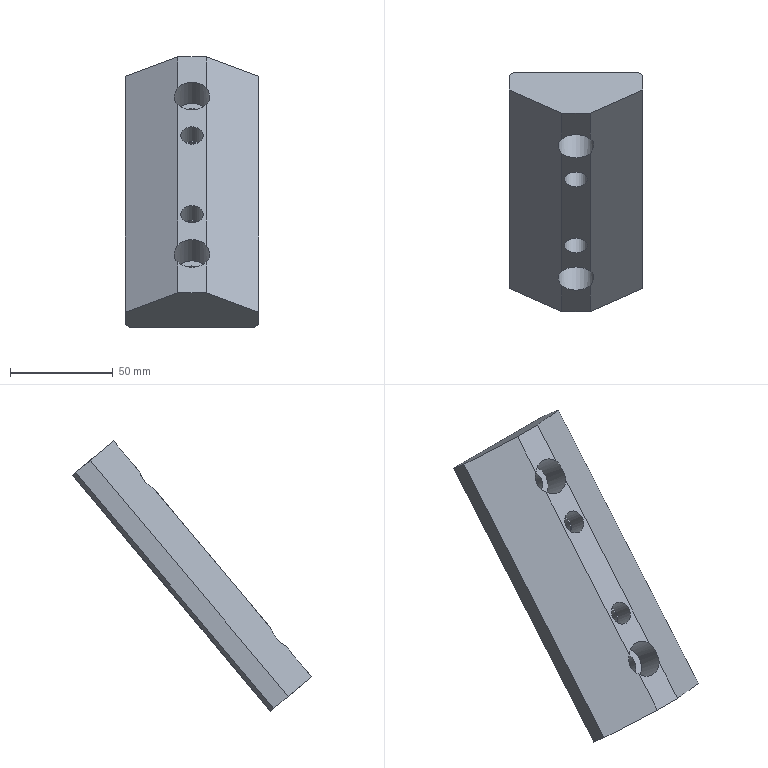Part | NX | features solid 2 | 1 solid | 24 faces | box 65 x 116.335 x 131.619 mm | volume 182247 mm3 | plane 16 | cylinder 8 | commonest cylinder face diameters 11 x4 10 x2 17.5 x2
STEP:
#1=CARTESIAN_POINT('',(-209.428,362.665,-180.748));
#2=VERTEX_POINT('',#1);
#3=CARTESIAN_POINT('',(-195.572,362.665,-180.748));
#4=VERTEX_POINT('',#3);
#5=CARTESIAN_POINT('',(-202.5,366.1,-176.654));
#6=DIRECTION('',(0.,-0.766,0.6428));
#7=DIRECTION('',(0.,0.6428,0.766));
#8=AXIS2_PLACEMENT_3D('',#5,#6,#7);
#9=CIRCLE('',#8,8.75);
#10=EDGE_CURVE('',#2,#4,#9,.T.);
#11=ORIENTED_EDGE('',*,*,#10,.F.);
#12=CARTESIAN_POINT('',(-209.428,350.031,-195.805));
#13=VERTEX_POINT('',#12);
#14=CARTESIAN_POINT('',(-209.428,350.031,-195.805));
#15=DIRECTION('',(0.,0.6428,0.766));
#16=VECTOR('',#15,1000.);
#17=LINE('',#14,#16);
#18=EDGE_CURVE('',#13,#2,#17,.T.);
#19=ORIENTED_EDGE('',*,*,#18,.F.);
#20=CARTESIAN_POINT('',(-195.572,350.031,-195.805));
#21=VERTEX_POINT('',#20);
#22=CARTESIAN_POINT('',(-195.572,350.031,-195.805));
#23=DIRECTION('',(-1.,0.,0.));
#24=VECTOR('',#23,1000.);
#25=LINE('',#22,#24);
#26=EDGE_CURVE('',#21,#13,#25,.T.);
#27=ORIENTED_EDGE('',*,*,#26,.F.);
#28=CARTESIAN_POINT('',(-195.572,350.031,-195.805));
#29=DIRECTION('',(0.,0.6428,0.766));
#30=VECTOR('',#29,1000.);
#31=LINE('',#28,#30);
#32=EDGE_CURVE('',#21,#4,#31,.T.);
#33=ORIENTED_EDGE('',*,*,#32,.T.);
#34=EDGE_LOOP('',(#11,#19,#27,#33));
#35=FACE_BOUND('',#34,.T.);
#36=CARTESIAN_POINT('',(-195.572,350.031,-195.805));
#37=DIRECTION('',(0.,-0.766,0.6428));
#38=DIRECTION('',(1.,0.,0.));
#39=AXIS2_PLACEMENT_3D('',#36,#37,#38);
#40=PLANE('',#39);
#41=ADVANCED_FACE('',(#35),#40,.T.);
#42=CARTESIAN_POINT('',(-202.5,385.705,-153.29));
#43=VERTEX_POINT('',#42);
#44=CARTESIAN_POINT('',(-202.5,382.17,-157.503));
#45=DIRECTION('',(0.,-0.766,0.6428));
#46=DIRECTION('',(0.,0.6428,0.766));
#47=AXIS2_PLACEMENT_3D('',#44,#45,#46);
#48=CIRCLE('',#47,5.5);
#49=EDGE_CURVE('',#43,#43,#48,.T.);
#50=ORIENTED_EDGE('',*,*,#49,.F.);
#51=EDGE_LOOP('',(#50));
#52=FACE_BOUND('',#51,.T.);
#53=CARTESIAN_POINT('',(-195.572,369.536,-172.56));
#54=VERTEX_POINT('',#53);
#55=CARTESIAN_POINT('',(-209.428,369.536,-172.56));
#56=VERTEX_POINT('',#55);
#57=CARTESIAN_POINT('',(-202.5,366.1,-176.654));
#58=DIRECTION('',(0.,-0.766,0.6428));
#59=DIRECTION('',(0.,0.6428,0.766));
#60=AXIS2_PLACEMENT_3D('',#57,#58,#59);
#61=CIRCLE('',#60,8.75);
#62=EDGE_CURVE('',#54,#56,#61,.T.);
#63=ORIENTED_EDGE('',*,*,#62,.F.);
#64=CARTESIAN_POINT('',(-195.572,426.944,-104.143));
#65=VERTEX_POINT('',#64);
#66=CARTESIAN_POINT('',(-195.572,350.031,-195.805));
#67=DIRECTION('',(0.,0.6428,0.766));
#68=VECTOR('',#67,1000.);
#69=LINE('',#66,#68);
#70=EDGE_CURVE('',#54,#65,#69,.T.);
#71=ORIENTED_EDGE('',*,*,#70,.T.);
#72=CARTESIAN_POINT('',(-209.428,426.944,-104.143));
#73=VERTEX_POINT('',#72);
#74=CARTESIAN_POINT('',(-202.5,430.379,-100.049));
#75=DIRECTION('',(0.,-0.766,0.6428));
#76=DIRECTION('',(0.,0.6428,0.766));
#77=AXIS2_PLACEMENT_3D('',#74,#75,#76);
#78=CIRCLE('',#77,8.75);
#79=EDGE_CURVE('',#73,#65,#78,.T.);
#80=ORIENTED_EDGE('',*,*,#79,.F.);
#81=CARTESIAN_POINT('',(-209.428,350.031,-195.805));
#82=DIRECTION('',(0.,0.6428,0.766));
#83=VECTOR('',#82,1000.);
#84=LINE('',#81,#83);
#85=EDGE_CURVE('',#56,#73,#84,.T.);
#86=ORIENTED_EDGE('',*,*,#85,.F.);
#87=EDGE_LOOP('',(#63,#71,#80,#86));
#88=FACE_BOUND('',#87,.T.);
#89=CARTESIAN_POINT('',(-202.5,417.845,-114.987));
#90=VERTEX_POINT('',#89);
#91=CARTESIAN_POINT('',(-202.5,414.309,-119.201));
#92=DIRECTION('',(0.,-0.766,0.6428));
#93=DIRECTION('',(0.,0.6428,0.766));
#94=AXIS2_PLACEMENT_3D('',#91,#92,#93);
#95=CIRCLE('',#94,5.5);
#96=EDGE_CURVE('',#90,#90,#95,.T.);
#97=ORIENTED_EDGE('',*,*,#96,.F.);
#98=EDGE_LOOP('',(#97));
#99=FACE_BOUND('',#98,.T.);
#100=CARTESIAN_POINT('',(-195.572,350.031,-195.805));
#101=DIRECTION('',(0.,-0.766,0.6428));
#102=DIRECTION('',(1.,0.,0.));
#103=AXIS2_PLACEMENT_3D('',#100,#101,#102);
#104=PLANE('',#103);
#105=ADVANCED_FACE('',(#52,#88,#99),#104,.T.);
#106=CARTESIAN_POINT('',(-202.5,363.036,-174.083));
#107=DIRECTION('',(0.5,0.6634,-0.5567));
#108=DIRECTION('',(-0.866,0.383,-0.3214));
#109=AXIS2_PLACEMENT_3D('',#106,#107,#108);
#110=ELLIPSE('',#109,10.104,8.75);
#111=EDGE_CURVE('',#2,#56,#110,.T.);
#112=ORIENTED_EDGE('',*,*,#111,.T.);
#113=ORIENTED_EDGE('',*,*,#85,.T.);
#114=CARTESIAN_POINT('',(-209.428,433.814,-95.955));
#115=VERTEX_POINT('',#114);
#116=CARTESIAN_POINT('',(-202.5,427.315,-97.478));
#117=DIRECTION('',(0.5,0.6634,-0.5567));
#118=DIRECTION('',(-0.866,0.383,-0.3214));
#119=AXIS2_PLACEMENT_3D('',#116,#117,#118);
#120=ELLIPSE('',#119,10.104,8.75);
#121=EDGE_CURVE('',#73,#115,#120,.T.);
#122=ORIENTED_EDGE('',*,*,#121,.T.);
#123=CARTESIAN_POINT('',(-209.428,446.449,-80.898));
#124=VERTEX_POINT('',#123);
#125=CARTESIAN_POINT('',(-209.428,350.031,-195.805));
#126=DIRECTION('',(0.,0.6428,0.766));
#127=VECTOR('',#126,1000.);
#128=LINE('',#125,#127);
#129=EDGE_CURVE('',#115,#124,#128,.T.);
#130=ORIENTED_EDGE('',*,*,#129,.T.);
#131=CARTESIAN_POINT('',(-235.,457.759,-90.388));
#132=VERTEX_POINT('',#131);
#133=CARTESIAN_POINT('',(-209.428,446.449,-80.898));
#134=DIRECTION('',(-0.866,0.383,-0.3214));
#135=VECTOR('',#134,1000.);
#136=LINE('',#133,#135);
#137=EDGE_CURVE('',#124,#132,#136,.T.);
#138=ORIENTED_EDGE('',*,*,#137,.T.);
#139=CARTESIAN_POINT('',(-235.,361.34,-205.295));
#140=VERTEX_POINT('',#139);
#141=CARTESIAN_POINT('',(-235.,361.34,-205.295));
#142=DIRECTION('',(0.,0.6428,0.766));
#143=VECTOR('',#142,1000.);
#144=LINE('',#141,#143);
#145=EDGE_CURVE('',#140,#132,#144,.T.);
#146=ORIENTED_EDGE('',*,*,#145,.F.);
#147=CARTESIAN_POINT('',(-209.428,350.031,-195.805));
#148=DIRECTION('',(-0.866,0.383,-0.3214));
#149=VECTOR('',#148,1000.);
#150=LINE('',#147,#149);
#151=EDGE_CURVE('',#13,#140,#150,.T.);
#152=ORIENTED_EDGE('',*,*,#151,.F.);
#153=ORIENTED_EDGE('',*,*,#18,.T.);
#154=EDGE_LOOP('',(#112,#113,#122,#130,#138,#146,#152,#153));
#155=FACE_BOUND('',#154,.T.);
#156=CARTESIAN_POINT('',(-209.428,350.031,-195.805));
#157=DIRECTION('',(-0.5,-0.6634,0.5567));
#158=DIRECTION('',(0.866,-0.383,0.3214));
#159=AXIS2_PLACEMENT_3D('',#156,#157,#158);
#160=PLANE('',#159);
#161=ADVANCED_FACE('',(#155),#160,.T.);
#162=CARTESIAN_POINT('',(-235.,368.416,-211.232));
#163=VERTEX_POINT('',#162);
#164=CARTESIAN_POINT('',(-235.,369.948,-212.517));
#165=DIRECTION('',(0.,-0.766,0.6428));
#166=VECTOR('',#165,1000.);
#167=LINE('',#164,#166);
#168=EDGE_CURVE('',#163,#140,#167,.T.);
#169=ORIENTED_EDGE('',*,*,#168,.T.);
#170=ORIENTED_EDGE('',*,*,#145,.T.);
#171=CARTESIAN_POINT('',(-235.,464.834,-96.325));
#172=VERTEX_POINT('',#171);
#173=CARTESIAN_POINT('',(-235.,466.366,-97.611));
#174=DIRECTION('',(0.,-0.766,0.6428));
#175=VECTOR('',#174,1000.);
#176=LINE('',#173,#175);
#177=EDGE_CURVE('',#172,#132,#176,.T.);
#178=ORIENTED_EDGE('',*,*,#177,.F.);
#179=CARTESIAN_POINT('',(-235.,368.416,-211.232));
#180=DIRECTION('',(0.,0.6428,0.766));
#181=VECTOR('',#180,1000.);
#182=LINE('',#179,#181);
#183=EDGE_CURVE('',#163,#172,#182,.T.);
#184=ORIENTED_EDGE('',*,*,#183,.F.);
#185=EDGE_LOOP('',(#169,#170,#178,#184));
#186=FACE_BOUND('',#185,.T.);
#187=CARTESIAN_POINT('',(-235.,369.948,-212.517));
#188=DIRECTION('',(1.,0.,0.));
#189=DIRECTION('',(0.,0.766,-0.6428));
#190=AXIS2_PLACEMENT_3D('',#187,#188,#189);
#191=PLANE('',#190);
#192=ADVANCED_FACE('',(#186),#191,.F.);
#193=CARTESIAN_POINT('',(-197.5,402.087,-174.215));
#194=VERTEX_POINT('',#193);
#195=CARTESIAN_POINT('',(-202.5,402.087,-174.215));
#196=DIRECTION('',(0.,0.766,-0.6428));
#197=DIRECTION('',(1.,0.,0.));
#198=AXIS2_PLACEMENT_3D('',#195,#196,#197);
#199=CIRCLE('',#198,5.);
#200=EDGE_CURVE('',#194,#194,#199,.T.);
#201=ORIENTED_EDGE('',*,*,#200,.F.);
#202=EDGE_LOOP('',(#201));
#203=FACE_BOUND('',#202,.T.);
#204=CARTESIAN_POINT('',(-197.,386.017,-193.366));
#205=VERTEX_POINT('',#204);
#206=CARTESIAN_POINT('',(-202.5,386.017,-193.366));
#207=DIRECTION('',(0.,0.766,-0.6428));
#208=DIRECTION('',(1.,0.,0.));
#209=AXIS2_PLACEMENT_3D('',#206,#207,#208);
#210=CIRCLE('',#209,5.5);
#211=EDGE_CURVE('',#205,#205,#210,.T.);
#212=ORIENTED_EDGE('',*,*,#211,.F.);
#213=EDGE_LOOP('',(#212));
#214=FACE_BOUND('',#213,.T.);
#215=CARTESIAN_POINT('',(-197.5,434.226,-135.913));
#216=VERTEX_POINT('',#215);
#217=CARTESIAN_POINT('',(-202.5,434.226,-135.913));
#218=DIRECTION('',(0.,0.766,-0.6428));
#219=DIRECTION('',(1.,0.,0.));
#220=AXIS2_PLACEMENT_3D('',#217,#218,#219);
#221=CIRCLE('',#220,5.);
#222=EDGE_CURVE('',#216,#216,#221,.T.);
#223=ORIENTED_EDGE('',*,*,#222,.F.);
#224=EDGE_LOOP('',(#223));
#225=FACE_BOUND('',#224,.T.);
#226=CARTESIAN_POINT('',(-197.,450.296,-116.762));
#227=VERTEX_POINT('',#226);
#228=CARTESIAN_POINT('',(-202.5,450.296,-116.762));
#229=DIRECTION('',(0.,0.766,-0.6428));
#230=DIRECTION('',(1.,0.,0.));
#231=AXIS2_PLACEMENT_3D('',#228,#229,#230);
#232=CIRCLE('',#231,5.5);
#233=EDGE_CURVE('',#227,#227,#232,.T.);
#234=ORIENTED_EDGE('',*,*,#233,.F.);
#235=EDGE_LOOP('',(#234));
#236=FACE_BOUND('',#235,.T.);
#237=CARTESIAN_POINT('',(-172.,466.366,-97.611));
#238=VERTEX_POINT('',#237);
#239=CARTESIAN_POINT('',(-233.,466.366,-97.611));
#240=VERTEX_POINT('',#239);
#241=CARTESIAN_POINT('',(-170.,466.366,-97.611));
#242=DIRECTION('',(-1.,0.,0.));
#243=VECTOR('',#242,1000.);
#244=LINE('',#241,#243);
#245=EDGE_CURVE('',#238,#240,#244,.T.);
#246=ORIENTED_EDGE('',*,*,#245,.F.);
#247=CARTESIAN_POINT('',(-172.,369.948,-212.517));
#248=VERTEX_POINT('',#247);
#249=CARTESIAN_POINT('',(-172.,369.948,-212.517));
#250=DIRECTION('',(0.,0.6428,0.766));
#251=VECTOR('',#250,1000.);
#252=LINE('',#249,#251);
#253=EDGE_CURVE('',#248,#238,#252,.T.);
#254=ORIENTED_EDGE('',*,*,#253,.F.);
#255=CARTESIAN_POINT('',(-233.,369.948,-212.517));
#256=VERTEX_POINT('',#255);
#257=CARTESIAN_POINT('',(-170.,369.948,-212.517));
#258=DIRECTION('',(-1.,0.,0.));
#259=VECTOR('',#258,1000.);
#260=LINE('',#257,#259);
#261=EDGE_CURVE('',#248,#256,#260,.T.);
#262=ORIENTED_EDGE('',*,*,#261,.T.);
#263=CARTESIAN_POINT('',(-233.,369.948,-212.517));
#264=DIRECTION('',(0.,-0.6428,-0.766));
#265=VECTOR('',#264,1000.);
#266=LINE('',#263,#265);
#267=EDGE_CURVE('',#240,#256,#266,.T.);
#268=ORIENTED_EDGE('',*,*,#267,.F.);
#269=EDGE_LOOP('',(#246,#254,#262,#268));
#270=FACE_BOUND('',#269,.T.);
#271=CARTESIAN_POINT('',(-170.,369.948,-212.517));
#272=DIRECTION('',(0.,-0.766,0.6428));
#273=DIRECTION('',(1.,0.,0.));
#274=AXIS2_PLACEMENT_3D('',#271,#272,#273);
#275=PLANE('',#274);
#276=ADVANCED_FACE('',(#203,#214,#225,#236,#270),#275,.F.);
#277=CARTESIAN_POINT('',(-170.,457.759,-90.388));
#278=VERTEX_POINT('',#277);
#279=CARTESIAN_POINT('',(-170.,464.834,-96.325));
#280=VERTEX_POINT('',#279);
#281=CARTESIAN_POINT('',(-170.,457.759,-90.388));
#282=DIRECTION('',(0.,0.766,-0.6428));
#283=VECTOR('',#282,1000.);
#284=LINE('',#281,#283);
#285=EDGE_CURVE('',#278,#280,#284,.T.);
#286=ORIENTED_EDGE('',*,*,#285,.F.);
#287=CARTESIAN_POINT('',(-170.,361.34,-205.295));
#288=VERTEX_POINT('',#287);
#289=CARTESIAN_POINT('',(-170.,361.34,-205.295));
#290=DIRECTION('',(0.,0.6428,0.766));
#291=VECTOR('',#290,1000.);
#292=LINE('',#289,#291);
#293=EDGE_CURVE('',#288,#278,#292,.T.);
#294=ORIENTED_EDGE('',*,*,#293,.F.);
#295=CARTESIAN_POINT('',(-170.,368.416,-211.232));
#296=VERTEX_POINT('',#295);
#297=CARTESIAN_POINT('',(-170.,361.34,-205.295));
#298=DIRECTION('',(0.,0.766,-0.6428));
#299=VECTOR('',#298,1000.);
#300=LINE('',#297,#299);
#301=EDGE_CURVE('',#288,#296,#300,.T.);
#302=ORIENTED_EDGE('',*,*,#301,.T.);
#303=CARTESIAN_POINT('',(-170.,368.416,-211.232));
#304=DIRECTION('',(0.,-0.6428,-0.766));
#305=VECTOR('',#304,1000.);
#306=LINE('',#303,#305);
#307=EDGE_CURVE('',#280,#296,#306,.T.);
#308=ORIENTED_EDGE('',*,*,#307,.F.);
#309=EDGE_LOOP('',(#286,#294,#302,#308));
#310=FACE_BOUND('',#309,.T.);
#311=CARTESIAN_POINT('',(-170.,361.34,-205.295));
#312=DIRECTION('',(-1.,0.,0.));
#313=DIRECTION('',(0.,-0.766,0.6428));
#314=AXIS2_PLACEMENT_3D('',#311,#312,#313);
#315=PLANE('',#314);
#316=ADVANCED_FACE('',(#310),#315,.F.);
#317=CARTESIAN_POINT('',(-202.5,363.036,-174.083));
#318=DIRECTION('',(-0.5,0.6634,-0.5567));
#319=DIRECTION('',(0.866,0.383,-0.3214));
#320=AXIS2_PLACEMENT_3D('',#317,#318,#319);
#321=ELLIPSE('',#320,10.104,8.75);
#322=EDGE_CURVE('',#54,#4,#321,.T.);
#323=ORIENTED_EDGE('',*,*,#322,.T.);
#324=ORIENTED_EDGE('',*,*,#32,.F.);
#325=CARTESIAN_POINT('',(-170.,361.34,-205.295));
#326=DIRECTION('',(-0.866,-0.383,0.3214));
#327=VECTOR('',#326,1000.);
#328=LINE('',#325,#327);
#329=EDGE_CURVE('',#288,#21,#328,.T.);
#330=ORIENTED_EDGE('',*,*,#329,.F.);
#331=ORIENTED_EDGE('',*,*,#293,.T.);
#332=CARTESIAN_POINT('',(-195.572,446.449,-80.898));
#333=VERTEX_POINT('',#332);
#334=CARTESIAN_POINT('',(-170.,457.759,-90.388));
#335=DIRECTION('',(-0.866,-0.383,0.3214));
#336=VECTOR('',#335,1000.);
#337=LINE('',#334,#336);
#338=EDGE_CURVE('',#278,#333,#337,.T.);
#339=ORIENTED_EDGE('',*,*,#338,.T.);
#340=CARTESIAN_POINT('',(-195.572,433.814,-95.955));
#341=VERTEX_POINT('',#340);
#342=CARTESIAN_POINT('',(-195.572,350.031,-195.805));
#343=DIRECTION('',(0.,0.6428,0.766));
#344=VECTOR('',#343,1000.);
#345=LINE('',#342,#344);
#346=EDGE_CURVE('',#341,#333,#345,.T.);
#347=ORIENTED_EDGE('',*,*,#346,.F.);
#348=CARTESIAN_POINT('',(-202.5,427.315,-97.478));
#349=DIRECTION('',(-0.5,0.6634,-0.5567));
#350=DIRECTION('',(0.866,0.383,-0.3214));
#351=AXIS2_PLACEMENT_3D('',#348,#349,#350);
#352=ELLIPSE('',#351,10.104,8.75);
#353=EDGE_CURVE('',#341,#65,#352,.T.);
#354=ORIENTED_EDGE('',*,*,#353,.T.);
#355=ORIENTED_EDGE('',*,*,#70,.F.);
#356=EDGE_LOOP('',(#323,#324,#330,#331,#339,#347,#354,#355));
#357=FACE_BOUND('',#356,.T.);
#358=CARTESIAN_POINT('',(-170.,361.34,-205.295));
#359=DIRECTION('',(0.5,-0.6634,0.5567));
#360=DIRECTION('',(0.866,0.383,-0.3214));
#361=AXIS2_PLACEMENT_3D('',#358,#359,#360);
#362=PLANE('',#361);
#363=ADVANCED_FACE('',(#357),#362,.T.);
#364=CARTESIAN_POINT('',(-202.5,430.379,-100.049));
#365=DIRECTION('',(0.,0.766,-0.6428));
#366=DIRECTION('',(1.,0.,0.));
#367=AXIS2_PLACEMENT_3D('',#364,#365,#366);
#368=CIRCLE('',#367,8.75);
#369=EDGE_CURVE('',#115,#341,#368,.T.);
#370=ORIENTED_EDGE('',*,*,#369,.T.);
#371=ORIENTED_EDGE('',*,*,#346,.T.);
#372=CARTESIAN_POINT('',(-195.572,446.449,-80.898));
#373=DIRECTION('',(-1.,0.,0.));
#374=VECTOR('',#373,1000.);
#375=LINE('',#372,#374);
#376=EDGE_CURVE('',#333,#124,#375,.T.);
#377=ORIENTED_EDGE('',*,*,#376,.T.);
#378=ORIENTED_EDGE('',*,*,#129,.F.);
#379=EDGE_LOOP('',(#370,#371,#377,#378));
#380=FACE_BOUND('',#379,.T.);
#381=CARTESIAN_POINT('',(-195.572,350.031,-195.805));
#382=DIRECTION('',(0.,-0.766,0.6428));
#383=DIRECTION('',(1.,0.,0.));
#384=AXIS2_PLACEMENT_3D('',#381,#382,#383);
#385=PLANE('',#384);
#386=ADVANCED_FACE('',(#380),#385,.T.);
#387=ORIENTED_EDGE('',*,*,#261,.F.);
#388=CARTESIAN_POINT('',(-172.25,370.139,-212.678));
#389=DIRECTION('',(0.7071,-0.5417,0.4545));
#390=VECTOR('',#389,1000.);
#391=LINE('',#388,#390);
#392=EDGE_CURVE('',#296,#248,#391,.F.);
#393=ORIENTED_EDGE('',*,*,#392,.F.);
#394=ORIENTED_EDGE('',*,*,#301,.F.);
#395=ORIENTED_EDGE('',*,*,#329,.T.);
#396=ORIENTED_EDGE('',*,*,#26,.T.);
#397=ORIENTED_EDGE('',*,*,#151,.T.);
#398=ORIENTED_EDGE('',*,*,#168,.F.);
#399=CARTESIAN_POINT('',(-232.75,370.139,-212.678));
#400=DIRECTION('',(0.7071,0.5417,-0.4545));
#401=VECTOR('',#400,1000.);
#402=LINE('',#399,#401);
#403=EDGE_CURVE('',#256,#163,#402,.F.);
#404=ORIENTED_EDGE('',*,*,#403,.F.);
#405=EDGE_LOOP('',(#387,#393,#394,#395,#396,#397,#398,#404));
#406=FACE_BOUND('',#405,.T.);
#407=CARTESIAN_POINT('',(-202.5,346.966,-193.234));
#408=DIRECTION('',(0.,-0.6428,-0.766));
#409=DIRECTION('',(0.,0.766,-0.6428));
#410=AXIS2_PLACEMENT_3D('',#407,#408,#409);
#411=PLANE('',#410);
#412=ADVANCED_FACE('',(#406),#411,.T.);
#413=ORIENTED_EDGE('',*,*,#177,.T.);
#414=ORIENTED_EDGE('',*,*,#137,.F.);
#415=ORIENTED_EDGE('',*,*,#376,.F.);
#416=ORIENTED_EDGE('',*,*,#338,.F.);
#417=ORIENTED_EDGE('',*,*,#285,.T.);
#418=CARTESIAN_POINT('',(-172.,466.366,-97.611));
#419=DIRECTION('',(-0.7071,0.5417,-0.4545));
#420=VECTOR('',#419,1000.);
#421=LINE('',#418,#420);
#422=EDGE_CURVE('',#238,#280,#421,.F.);
#423=ORIENTED_EDGE('',*,*,#422,.F.);
#424=ORIENTED_EDGE('',*,*,#245,.T.);
#425=CARTESIAN_POINT('',(-235.,464.834,-96.325));
#426=DIRECTION('',(-0.7071,-0.5417,0.4545));
#427=VECTOR('',#426,1000.);
#428=LINE('',#425,#427);
#429=EDGE_CURVE('',#172,#240,#428,.F.);
#430=ORIENTED_EDGE('',*,*,#429,.F.);
#431=EDGE_LOOP('',(#413,#414,#415,#416,#417,#423,#424,#430));
#432=FACE_BOUND('',#431,.T.);
#433=CARTESIAN_POINT('',(-202.5,443.385,-78.327));
#434=DIRECTION('',(0.,-0.6428,-0.766));
#435=DIRECTION('',(0.,0.766,-0.6428));
#436=AXIS2_PLACEMENT_3D('',#433,#434,#435);
#437=PLANE('',#436);
#438=ADVANCED_FACE('',(#432),#437,.F.);
#439=CARTESIAN_POINT('',(-202.5,446.171,-106.121));
#440=VERTEX_POINT('',#439);
#441=CARTESIAN_POINT('',(-202.5,442.636,-110.334));
#442=DIRECTION('',(0.,-0.766,0.6428));
#443=DIRECTION('',(0.,0.6428,0.766));
#444=AXIS2_PLACEMENT_3D('',#441,#442,#443);
#445=CIRCLE('',#444,5.5);
#446=EDGE_CURVE('',#440,#440,#445,.T.);
#447=ORIENTED_EDGE('',*,*,#446,.T.);
#448=EDGE_LOOP('',(#447));
#449=FACE_BOUND('',#448,.T.);
#450=ORIENTED_EDGE('',*,*,#233,.T.);
#451=EDGE_LOOP('',(#450));
#452=FACE_BOUND('',#451,.T.);
#453=CARTESIAN_POINT('',(-202.5,453.36,-119.333));
#454=DIRECTION('',(0.,0.766,-0.6428));
#455=DIRECTION('',(0.,0.6428,0.766));
#456=AXIS2_PLACEMENT_3D('',#453,#454,#455);
#457=CYLINDRICAL_SURFACE('',#456,5.5);
#458=ADVANCED_FACE('',(#449,#452),#457,.F.);
#459=ORIENTED_EDGE('',*,*,#446,.F.);
#460=EDGE_LOOP('',(#459));
#461=FACE_BOUND('',#460,.T.);
#462=CARTESIAN_POINT('',(-202.5,448.26,-103.631));
#463=VERTEX_POINT('',#462);
#464=CARTESIAN_POINT('',(-202.5,442.636,-110.334));
#465=DIRECTION('',(0.,-0.766,0.6428));
#466=DIRECTION('',(0.,0.6428,0.766));
#467=AXIS2_PLACEMENT_3D('',#464,#465,#466);
#468=CIRCLE('',#467,8.75);
#469=EDGE_CURVE('',#463,#463,#468,.T.);
#470=ORIENTED_EDGE('',*,*,#469,.T.);
#471=EDGE_LOOP('',(#470));
#472=FACE_BOUND('',#471,.T.);
#473=CARTESIAN_POINT('',(-202.5,442.636,-110.334));
#474=DIRECTION('',(0.,0.766,-0.6428));
#475=DIRECTION('',(0.,0.6428,0.766));
#476=AXIS2_PLACEMENT_3D('',#473,#474,#475);
#477=PLANE('',#476);
#478=ADVANCED_FACE('',(#461,#472),#477,.F.);
#479=ORIENTED_EDGE('',*,*,#121,.F.);
#480=ORIENTED_EDGE('',*,*,#79,.T.);
#481=ORIENTED_EDGE('',*,*,#353,.F.);
#482=ORIENTED_EDGE('',*,*,#369,.F.);
#483=EDGE_LOOP('',(#479,#480,#481,#482));
#484=FACE_BOUND('',#483,.T.);
#485=ORIENTED_EDGE('',*,*,#469,.F.);
#486=EDGE_LOOP('',(#485));
#487=FACE_BOUND('',#486,.T.);
#488=CARTESIAN_POINT('',(-202.5,430.379,-100.049));
#489=DIRECTION('',(0.,0.766,-0.6428));
#490=DIRECTION('',(0.,0.6428,0.766));
#491=AXIS2_PLACEMENT_3D('',#488,#489,#490);
#492=CYLINDRICAL_SURFACE('',#491,8.75);
#493=ADVANCED_FACE('',(#484,#487),#492,.F.);
#494=CARTESIAN_POINT('',(-202.5,425.95,-122.441));
#495=VERTEX_POINT('',#494);
#496=CARTESIAN_POINT('',(-202.5,422.736,-126.271));
#497=DIRECTION('',(0.,-0.766,0.6428));
#498=DIRECTION('',(0.,0.6428,0.766));
#499=AXIS2_PLACEMENT_3D('',#496,#497,#498);
#500=CIRCLE('',#499,5.);
#501=EDGE_CURVE('',#495,#495,#500,.T.);
#502=ORIENTED_EDGE('',*,*,#501,.T.);
#503=EDGE_LOOP('',(#502));
#504=FACE_BOUND('',#503,.T.);
#505=ORIENTED_EDGE('',*,*,#222,.T.);
#506=EDGE_LOOP('',(#505));
#507=FACE_BOUND('',#506,.T.);
#508=CARTESIAN_POINT('',(-202.5,437.291,-138.484));
#509=DIRECTION('',(0.,0.766,-0.6428));
#510=DIRECTION('',(0.,0.6428,0.766));
#511=AXIS2_PLACEMENT_3D('',#508,#509,#510);
#512=CYLINDRICAL_SURFACE('',#511,5.);
#513=ADVANCED_FACE('',(#504,#507),#512,.F.);
#514=ORIENTED_EDGE('',*,*,#501,.F.);
#515=EDGE_LOOP('',(#514));
#516=FACE_BOUND('',#515,.T.);
#517=CARTESIAN_POINT('',(-202.5,426.271,-122.058));
#518=VERTEX_POINT('',#517);
#519=CARTESIAN_POINT('',(-202.5,422.736,-126.271));
#520=DIRECTION('',(0.,-0.766,0.6428));
#521=DIRECTION('',(0.,0.6428,0.766));
#522=AXIS2_PLACEMENT_3D('',#519,#520,#521);
#523=CIRCLE('',#522,5.5);
#524=EDGE_CURVE('',#518,#518,#523,.T.);
#525=ORIENTED_EDGE('',*,*,#524,.T.);
#526=EDGE_LOOP('',(#525));
#527=FACE_BOUND('',#526,.T.);
#528=CARTESIAN_POINT('',(-202.5,422.736,-126.271));
#529=DIRECTION('',(0.,0.766,-0.6428));
#530=DIRECTION('',(0.,0.6428,0.766));
#531=AXIS2_PLACEMENT_3D('',#528,#529,#530);
#532=PLANE('',#531);
#533=ADVANCED_FACE('',(#516,#527),#532,.F.);
#534=ORIENTED_EDGE('',*,*,#524,.F.);
#535=EDGE_LOOP('',(#534));
#536=FACE_BOUND('',#535,.T.);
#537=ORIENTED_EDGE('',*,*,#96,.T.);
#538=EDGE_LOOP('',(#537));
#539=FACE_BOUND('',#538,.T.);
#540=CARTESIAN_POINT('',(-202.5,414.309,-119.201));
#541=DIRECTION('',(0.,0.766,-0.6428));
#542=DIRECTION('',(0.,0.6428,0.766));
#543=AXIS2_PLACEMENT_3D('',#540,#541,#542);
#544=CYLINDRICAL_SURFACE('',#543,5.5);
#545=ADVANCED_FACE('',(#536,#539),#544,.F.);
#546=CARTESIAN_POINT('',(-202.5,381.892,-182.725));
#547=VERTEX_POINT('',#546);
#548=CARTESIAN_POINT('',(-202.5,378.357,-186.938));
#549=DIRECTION('',(0.,-0.766,0.6428));
#550=DIRECTION('',(0.,0.6428,0.766));
#551=AXIS2_PLACEMENT_3D('',#548,#549,#550);
#552=CIRCLE('',#551,5.5);
#553=EDGE_CURVE('',#547,#547,#552,.T.);
#554=ORIENTED_EDGE('',*,*,#553,.T.);
#555=EDGE_LOOP('',(#554));
#556=FACE_BOUND('',#555,.T.);
#557=ORIENTED_EDGE('',*,*,#211,.T.);
#558=EDGE_LOOP('',(#557));
#559=FACE_BOUND('',#558,.T.);
#560=CARTESIAN_POINT('',(-202.5,389.082,-195.938));
#561=DIRECTION('',(0.,0.766,-0.6428));
#562=DIRECTION('',(0.,0.6428,0.766));
#563=AXIS2_PLACEMENT_3D('',#560,#561,#562);
#564=CYLINDRICAL_SURFACE('',#563,5.5);
#565=ADVANCED_FACE('',(#556,#559),#564,.F.);
#566=ORIENTED_EDGE('',*,*,#553,.F.);
#567=EDGE_LOOP('',(#566));
#568=FACE_BOUND('',#567,.T.);
#569=CARTESIAN_POINT('',(-202.5,383.981,-180.236));
#570=VERTEX_POINT('',#569);
#571=CARTESIAN_POINT('',(-202.5,378.357,-186.938));
#572=DIRECTION('',(0.,-0.766,0.6428));
#573=DIRECTION('',(0.,0.6428,0.766));
#574=AXIS2_PLACEMENT_3D('',#571,#572,#573);
#575=CIRCLE('',#574,8.75);
#576=EDGE_CURVE('',#570,#570,#575,.T.);
#577=ORIENTED_EDGE('',*,*,#576,.T.);
#578=EDGE_LOOP('',(#577));
#579=FACE_BOUND('',#578,.T.);
#580=CARTESIAN_POINT('',(-202.5,378.357,-186.938));
#581=DIRECTION('',(0.,0.766,-0.6428));
#582=DIRECTION('',(0.,0.6428,0.766));
#583=AXIS2_PLACEMENT_3D('',#580,#581,#582);
#584=PLANE('',#583);
#585=ADVANCED_FACE('',(#568,#579),#584,.F.);
#586=ORIENTED_EDGE('',*,*,#111,.F.);
#587=ORIENTED_EDGE('',*,*,#10,.T.);
#588=ORIENTED_EDGE('',*,*,#322,.F.);
#589=ORIENTED_EDGE('',*,*,#62,.T.);
#590=EDGE_LOOP('',(#586,#587,#588,#589));
#591=FACE_BOUND('',#590,.T.);
#592=ORIENTED_EDGE('',*,*,#576,.F.);
#593=EDGE_LOOP('',(#592));
#594=FACE_BOUND('',#593,.T.);
#595=CARTESIAN_POINT('',(-202.5,366.1,-176.654));
#596=DIRECTION('',(0.,0.766,-0.6428));
#597=DIRECTION('',(0.,0.6428,0.766));
#598=AXIS2_PLACEMENT_3D('',#595,#596,#597);
#599=CYLINDRICAL_SURFACE('',#598,8.75);
#600=ADVANCED_FACE('',(#591,#594),#599,.F.);
#601=CARTESIAN_POINT('',(-202.5,393.81,-160.743));
#602=VERTEX_POINT('',#601);
#603=CARTESIAN_POINT('',(-202.5,390.596,-164.573));
#604=DIRECTION('',(0.,-0.766,0.6428));
#605=DIRECTION('',(0.,0.6428,0.766));
#606=AXIS2_PLACEMENT_3D('',#603,#604,#605);
#607=CIRCLE('',#606,5.);
#608=EDGE_CURVE('',#602,#602,#607,.T.);
#609=ORIENTED_EDGE('',*,*,#608,.T.);
#610=EDGE_LOOP('',(#609));
#611=FACE_BOUND('',#610,.T.);
#612=ORIENTED_EDGE('',*,*,#200,.T.);
#613=EDGE_LOOP('',(#612));
#614=FACE_BOUND('',#613,.T.);
#615=CARTESIAN_POINT('',(-202.5,405.151,-176.786));
#616=DIRECTION('',(0.,0.766,-0.6428));
#617=DIRECTION('',(0.,0.6428,0.766));
#618=AXIS2_PLACEMENT_3D('',#615,#616,#617);
#619=CYLINDRICAL_SURFACE('',#618,5.);
#620=ADVANCED_FACE('',(#611,#614),#619,.F.);
#621=ORIENTED_EDGE('',*,*,#608,.F.);
#622=EDGE_LOOP('',(#621));
#623=FACE_BOUND('',#622,.T.);
#624=CARTESIAN_POINT('',(-202.5,394.132,-160.36));
#625=VERTEX_POINT('',#624);
#626=CARTESIAN_POINT('',(-202.5,390.596,-164.573));
#627=DIRECTION('',(0.,-0.766,0.6428));
#628=DIRECTION('',(0.,0.6428,0.766));
#629=AXIS2_PLACEMENT_3D('',#626,#627,#628);
#630=CIRCLE('',#629,5.5);
#631=EDGE_CURVE('',#625,#625,#630,.T.);
#632=ORIENTED_EDGE('',*,*,#631,.T.);
#633=EDGE_LOOP('',(#632));
#634=FACE_BOUND('',#633,.T.);
#635=CARTESIAN_POINT('',(-202.5,390.596,-164.573));
#636=DIRECTION('',(0.,0.766,-0.6428));
#637=DIRECTION('',(0.,0.6428,0.766));
#638=AXIS2_PLACEMENT_3D('',#635,#636,#637);
#639=PLANE('',#638);
#640=ADVANCED_FACE('',(#623,#634),#639,.F.);
#641=ORIENTED_EDGE('',*,*,#631,.F.);
#642=EDGE_LOOP('',(#641));
#643=FACE_BOUND('',#642,.T.);
#644=ORIENTED_EDGE('',*,*,#49,.T.);
#645=EDGE_LOOP('',(#644));
#646=FACE_BOUND('',#645,.T.);
#647=CARTESIAN_POINT('',(-202.5,382.17,-157.503));
#648=DIRECTION('',(0.,0.766,-0.6428));
#649=DIRECTION('',(0.,0.6428,0.766));
#650=AXIS2_PLACEMENT_3D('',#647,#648,#649);
#651=CYLINDRICAL_SURFACE('',#650,5.5);
#652=ADVANCED_FACE('',(#643,#646),#651,.F.);
#653=ORIENTED_EDGE('',*,*,#403,.T.);
#654=ORIENTED_EDGE('',*,*,#183,.T.);
#655=ORIENTED_EDGE('',*,*,#429,.T.);
#656=ORIENTED_EDGE('',*,*,#267,.T.);
#657=EDGE_LOOP('',(#653,#654,#655,#656));
#658=FACE_BOUND('',#657,.T.);
#659=CARTESIAN_POINT('',(-235.,368.416,-211.232));
#660=DIRECTION('',(0.7071,-0.5417,0.4545));
#661=DIRECTION('',(0.7071,0.5417,-0.4545));
#662=AXIS2_PLACEMENT_3D('',#659,#660,#661);
#663=PLANE('',#662);
#664=ADVANCED_FACE('',(#658),#663,.F.);
#665=ORIENTED_EDGE('',*,*,#392,.T.);
#666=ORIENTED_EDGE('',*,*,#253,.T.);
#667=ORIENTED_EDGE('',*,*,#422,.T.);
#668=ORIENTED_EDGE('',*,*,#307,.T.);
#669=EDGE_LOOP('',(#665,#666,#667,#668));
#670=FACE_BOUND('',#669,.T.);
#671=CARTESIAN_POINT('',(-172.,369.948,-212.517));
#672=DIRECTION('',(-0.7071,-0.5417,0.4545));
#673=DIRECTION('',(0.7071,-0.5417,0.4545));
#674=AXIS2_PLACEMENT_3D('',#671,#672,#673);
#675=PLANE('',#674);
#676=ADVANCED_FACE('',(#670),#675,.F.);
#677=CLOSED_SHELL('',(#41,#105,#161,#192,#276,#316,#363,#386,#412,#438,#458,#478,#493,#513,#533,#545,#565,#585,#600,#620,#640,#652,#664,#676));
#678=MANIFOLD_SOLID_BREP('',#677);
#679=(LENGTH_UNIT()NAMED_UNIT(*)SI_UNIT(.MILLI.,.METRE.));
#680=UNCERTAINTY_MEASURE_WITH_UNIT(LENGTH_MEASURE(0.00001),#679,'','');
#681=(NAMED_UNIT(*)PLANE_ANGLE_UNIT()SI_UNIT($,.RADIAN.));
#682=(NAMED_UNIT(*)SI_UNIT($,.STERADIAN.)SOLID_ANGLE_UNIT());
#683=(GEOMETRIC_REPRESENTATION_CONTEXT(3)GLOBAL_UNCERTAINTY_ASSIGNED_CONTEXT((#680))GLOBAL_UNIT_ASSIGNED_CONTEXT((#679,#681,#682))REPRESENTATION_CONTEXT('',''));
#684=ADVANCED_BREP_SHAPE_REPRESENTATION('',(#678),#683);